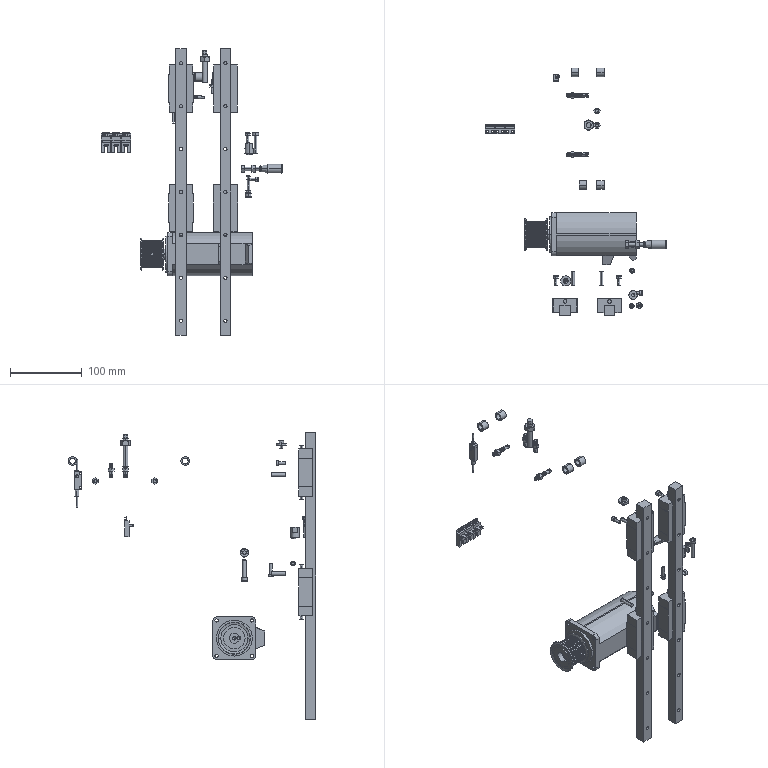Part | NX | 45 solids | 2676 faces | box 253.4 x 345.83 x 400 mm | volume 730030 mm3 | plane 1757 | cylinder 725 | cone 140 | spline 44 | sphere 6 | torus 4 | commonest cylinder face diameters 5 x203 0.5 x52 6.55 x52 1.1 x48 37.24 x48 4.5 x36